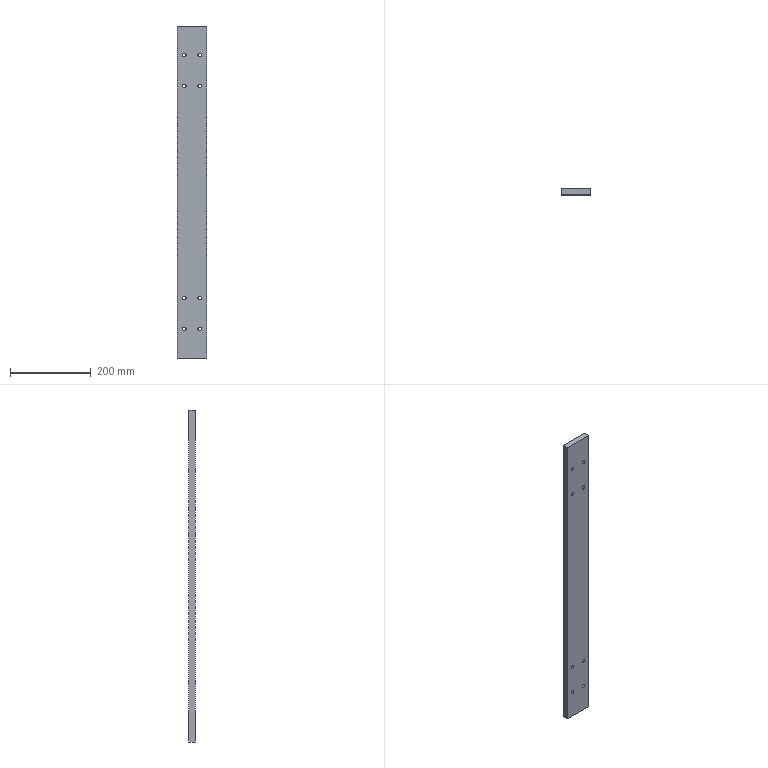Part | STEP file | Middle link plate | 1 solid | 22 faces | box 74 x 15 x 820 mm | volume 903391 mm3 | cylinder 16 | plane 6 | commonest cylinder face diameters 8.5 x16